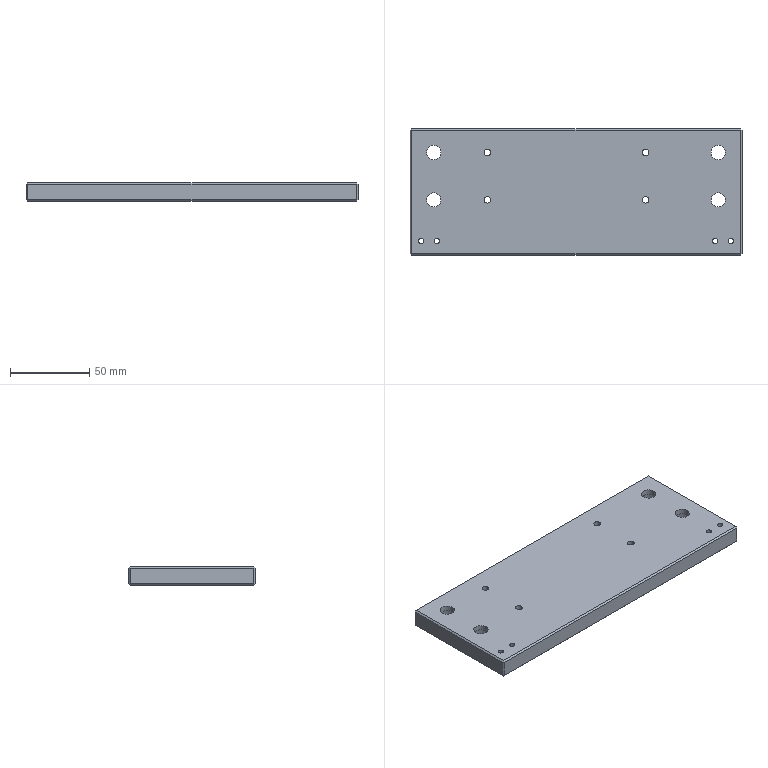Part | STEP file | 02-01 module support plate A | 1 solid | 70 faces | box 210 x 80 x 12 mm | volume 192896 mm3 | cylinder 36 | plane 30 | cone 4 | commonest cylinder face diameters 3.3 x8 4.2 x8 9 x8 15 x8 2.5 x4